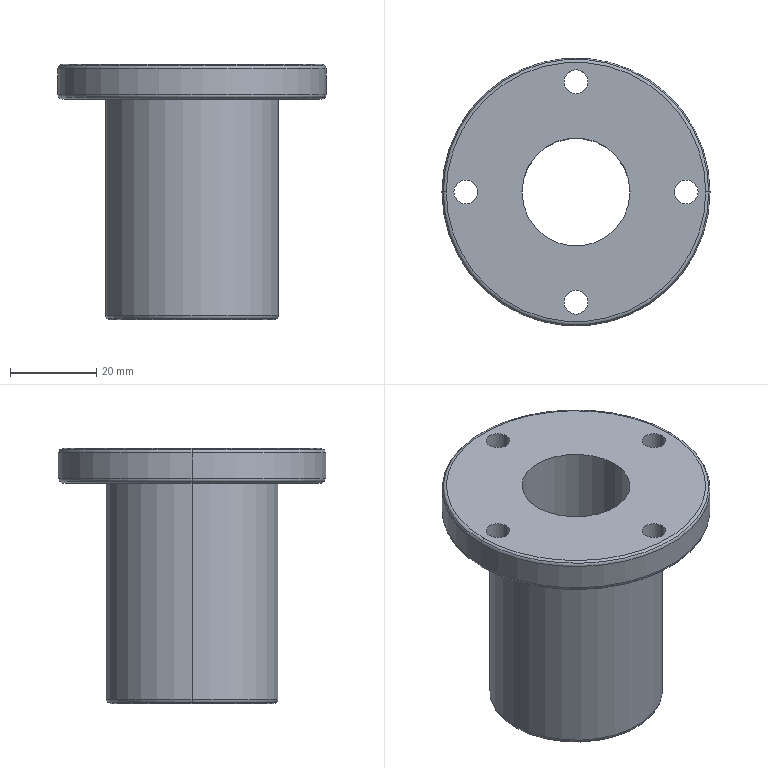Part | NX | features BREP 1 | 1 solid | 65 faces | box 62 x 62 x 59 mm | volume 58368 mm3 | plane 27 | cylinder 20 | torus 12 | cone 6 | commonest cylinder face diameters 5.5 x8 8.5 x6 25 x2 40 x2 62 x2